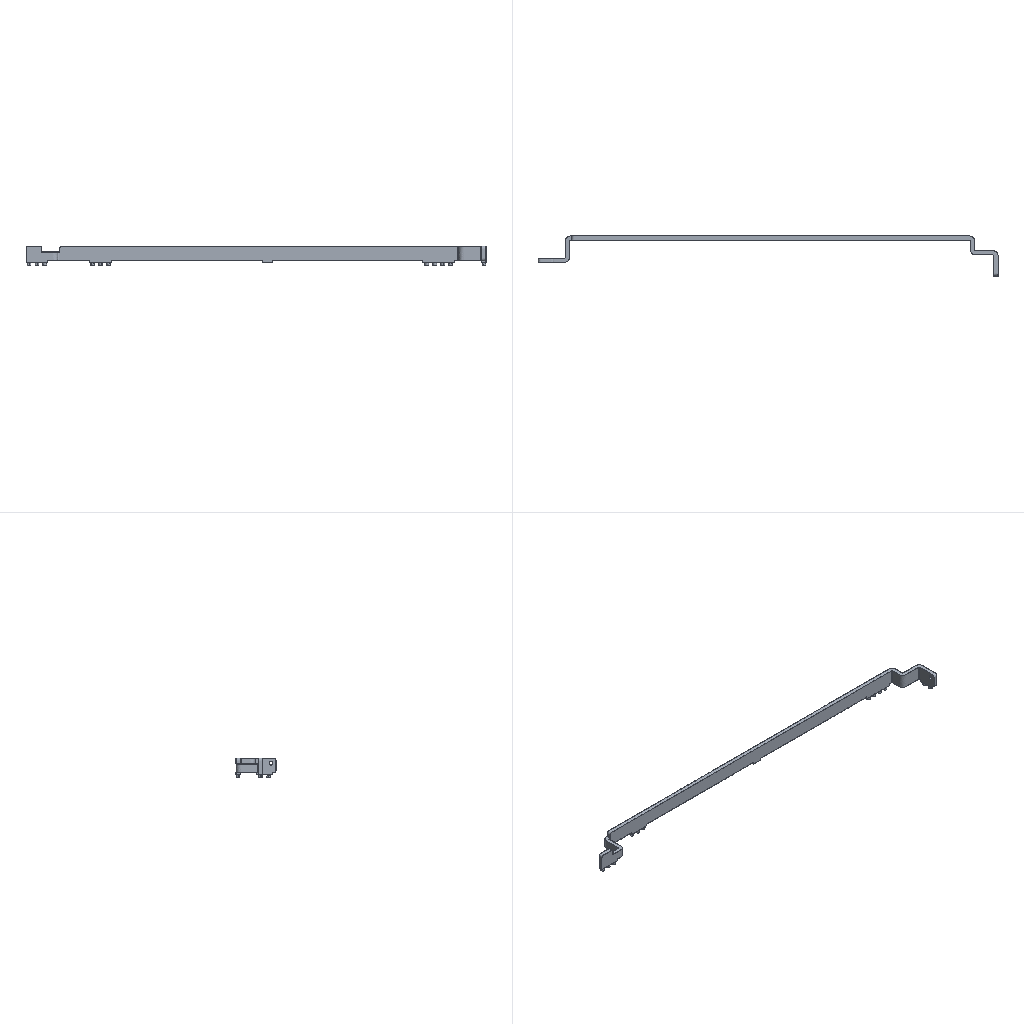Simulation study | ansys workbench
Set-up summary:
category,name,step,type,value,unit,region
solver,ansys_workbench
units,um-kg-s,,stated,"/units,uMKS"
analysis,LS1,,steady-state thermal
load_step,LS1,LS1,steady-state thermal,nsubst=1; time=1
mesh,nodes,,,149873
mesh,elements,,,151301
element_type,SOLID291,,,45869
element_type,227,,,30168
element_type,TARGE170,,,29349
element_type,CONTA174,,,29349
element_type,SURF152,,,16566
material,?,,E,3780,MPa
material,?,,nu,0.35
material,?,,density,1.16e-15,kg um^-3
material,?,,conductivity,200000,pW um^-1 C^-1
material,Copper Alloy,,E,110000,MPa
material,Copper Alloy,,nu,0.34
material,Copper Alloy,,density,8.3e-15,kg um^-3
material,Copper Alloy,,conductivity,4.01e+08,pW um^-1 C^-1
material,Copper Alloy,,specific_heat,3.85e+14,pJ kg^-1 C^-1
material,Copper Alloy,,cte,1.8e-05,C^-1
material,Copper Alloy,,permeability,1
material,Copper Alloy,,resistivity,1.548e-14
load,,LS1,force,0 [n=2],,node list
load,"Create ""______""",LS1,convection,20,,SURF152 #5
bc,,LS1,prescribed volt,[dofs=VOLT],,node list
contact,Contact Region,,bonded (always),element=CONTA174
constraint,ce,,,948
named_set,_CM38,,node,455
Ansys APDL input file, long lists of numbers shortened:
/batch
/config,noeldb,1     ! force off writing results to database
*get,_wallstrt,active,,time,wall
! ANSYS input file written by Workbench version 2021 R2
! File used for geometry attach:
/title,wbnew--______ (A5)
! ****** Begin Custom Load Command Snippet ******
/COM, ACT Extensions:
/COM,     LSDYNA, 2021.1
/COM,
! ****** End   Custom Load Command Snippet ******
*DIM,_wb_ProjectScratch_dir,string,248
_wb_ProjectScratch_dir(1) = ''
*DIM,_wb_SolverFiles_dir,string,248
_wb_SolverFiles_dir(1) = ''
*DIM,_wb_userfiles_dir,string,248
_wb_userfiles_dir(1) = ''
/com,--- Data in consistent uMKS units. See Solving Units in the help system for more information.
/units,uMKS
/nopr
/wb,file,start              !  signify a WB generated input file
/prep7
! Turn off shape checking because checks already performed inside WB mesher.
! See help system for more information.
SHPP,OFF,,NOWARN
ncnv,1,1e9             ! uMKS system, Increase DOF limit to 1e9
/nolist
etcon,set             ! allow ANSYS to choose best KEYOP's for 180x elements, resets any applicable keyopt to MAPDL defaults
/com,*********** Nodes for the whole assembly ***********
nblock,3,,164860
(1i9,3e20.9e3)
        1     8.444409090E+04     1.904694042E+04     7.400000000E+03
! (149872 more lines like these left out)
-1
/wb,elem,start            !  set before creation of elements
/com,*********** Elements for Body 1 "i24A7-2S - COATING" ***********
et,1,291
eblock,19,solid,,45869
(19i9)
        1        1        1        1        0        0        0        0       10        0    30169    57363    72055    62480    57436    73682   107343    73679    73678
! (91737 more lines like these left out)
-1
/com,*********** Elements for Body 2 "i24A7-2S" ***********
et,2,227,110
eblock,19,solid,,30168
(19i9)
        2        2        2        2        0        0        0        0       10        0        1     3967     9597     8304     8315    32140    53754    32137    32138
! (60335 more lines like these left out)
-1
/wb,elem,end               !  done creating elements
/com,*********** Send User Defined Coordinate System(s) ***********
csys,0
toffst,273.15,  ! Temperature offset from absolute zero
/com,*********** Set Reference Temperature ***********
tref,22.
/wb,mat,start              !  starting to send materials
/com,*********** Send Materials ***********
MP,DENS,1,1.16e-15,	! kg um^-3
MP,EX,1,3780,	! MPa
MP,NUXY,1,0.35,
MP,KXX,1,200000,	! pW um^-1 C^-1
Temperature = 'TEMP' ! Temperature
MP,DENS,2,8.3e-15,	! kg um^-3
MP,ALPX,2,1.8e-05,	! C^-1
MP,C,2,385000000000000,	! pJ kg^-1 C^-1
MP,KXX,2,401000000,	! pW um^-1 C^-1
MPTEMP,,,,,,,,
MPTEMP,1,0
MPTEMP,2,20
MPTEMP,3,100
MPDATA,RSVX,2, ,1.548e-14,1.694e-14,2.277e-14,	! Tohm um
MPTEMP,,,,,,,,
MP,EX,2,110000,	! MPa
MP,NUXY,2,0.34,
MP,MURX,2,1,
/wb,mat,end                !  done sending materials
!************************* Model Summary ********************
!i24A7-2S - COATING,	环氧树脂,	matid,	1
!i24A7-2S,	铜合金,	matid,	2
!************************* End Model Summary ********************
! get the diagonal of the bounding box. Needed later for other things
*get,_xmin,node,,mnloc,x
*get,_ymin,node,,mnloc,y
*get,_zmin,node,,mnloc,z
*get,_xmax,node,,mxloc,x
*get,_ymax,node,,mxloc,y
*get,_zmax,node,,mxloc,z
_ASMDIAG=(_xmax-_xmin)*(_xmax-_xmin)+(_ymax-_ymin)*(_ymax-_ymin)+(_zmax-_zmin)*(_zmax-_zmin)
_ASMDIAG=SQRT(_ASMDIAG)
/wb,contact,start          !  starting to send contact
/com,*********** Create Contact "接触区域" ***********
/com,            Real Constant Set For Above Contact Is 4 & 3
*set,tid,4
*set,cid,3
r,tid
r,cid
et,tid,170
et,cid,174
eblock,10,,,15039
(15i9)
   122828        4        4        4        0    60070    60066    60071    60071    91609    91610    60071    91632
! (15038 more lines like these left out)
-1
eblock,10,,,15039
(15i9)
   137867        3        3        3        0    60070    60066    60071    60071    91609    91610    60071    91632
! (15038 more lines like these left out)
-1
eblock,10,,,14310
(15i9)
   152906        3        4        3        0      268      264      267      267    11334    11333      267    11360
! (14309 more lines like these left out)
-1
eblock,10,,,14310
(15i9)
   167216        4        3        4        0      268      264      267      267    11334    11333      267    11360
! (14309 more lines like these left out)
-1
keyo,cid,8,2               ! auto create asymmetric contact (from Program Controlled setting)
keyo,cid,10,0              ! adjust contact stiffness each NR iteration (from Program Controlled setting)
keyo,cid,12,5              ! bonded always
keyo,cid,18,1              ! small sliding turned on by application
keyo,cid,2,0               ! augmented Lagrange (from Program Controlled setting)
keyo,cid,4,0               ! on Gauss point (from Program Controlled setting)
keyo,cid,9,1               ! ignore initial gaps/penetration
keyo,cid,7,0               ! No Prediction
rmod,tid,3,10.      ! FKN
rmod,tid,5,0.       ! ICONT
rmod,tid,6,0.       ! PINB
rmod,tid,10,0.      ! CNOF
rmod,tid,12,0.      ! FKT
rmod,tid,36,29      ! WB DSID
rmod,cid,3,10.      ! FKN
rmod,cid,5,0.       ! ICONT
rmod,cid,6,0.       ! PINB
rmod,cid,10,0.      ! CNOF
rmod,cid,12,0.      ! FKT
rmod,cid,36,29      ! WB DSID
*set,_maxkxx,4010000000000.
rmod,cid,14,_maxkxx/_ASMDIAG         ! TCC, Divide by Length since Traction Based
rmod,tid,14,_maxkxx/_ASMDIAG      ! TCC, Divide by Length since Traction Based
keyo,cid,1,2     ! Pure thermal contact
nsel,all
esel,all
/wb,contact,end            !  done creating contacts
/golist
/wb,load,start             !  starting to send loads
/com,*********** Create Voltage "__" ***********
CMBLOCK,_CM38   ,NODE,      455
(8i10)
       140       141       142       143       144       145       146       147
! (56 more lines like these left out)
/com,*********** Create Current ***********
/com,*********** Create Current ***********
fcum,add                   ! add nodal forces up (needed in case have loads on the same edge,vertex)
fcum                       ! reset default on fcum command since done sending WB F loads
/com,*********** Create "______" ***********
et,5,152
eblock,10,,,16566
(15i9)
   181526        5        5        5        0    57519    57520    59741    59741    74470    74476    59741    74472
! (16565 more lines like these left out)
-1
esel,s,type,,5
keyop,5,8,2.
keyop,5,13,0
esel,all
/gst,on,on
fini
*get,_numnode,node,0,count
*get,_numelem,elem,0,count
*get, _MAXELEMNUM, elem, 0, NUM, MAX
*get, _MAXNODENUM, node, 0, NUM, MAX
*get, _MAXELEMTYPE, etyp, 0, NUM, MAX
*get, _MAXREALCONST, real, 0, NUM, MAX
/go
/wb,load,end               !  done creating loads
/com,--- Number of total nodes = %_numnode%
/com,--- Number of contact elements = 75264
/com,--- Number of spring elements = 0
/com,--- Number of bearing elements = 0
/com,--- Number of solid elements = 76037
/com,--- Number of condensed parts = 0
/com,--- Number of total elements = %_numelem%
*get,_wallbsol,active,,time,wall
/com,****************************************************************************
/com,*************************    SOLUTION       ********************************
/com,****************************************************************************
/solu
antype,0                   ! static analysis
!eqsl,sparse               ! using sparse solver which is default so no eqsl command needed
cntr,print,1               ! print out contact info and also make no initial contact an error
dmpoption,emat,no             ! Don't combine emat file for DANSYS
dmpoption,esav,no             ! Don't combine esav file for DANSYS
/com,****************************************************
/com,******************* SOLVE FOR LS 1 OF 1****************
d,_CM38,volt,0.
nsel,all
f,23,amps,140000000000000
ce,next,0.,23,volt,-1.,24,volt,1.
ce,next,0.,23,volt,-1.,25,volt,1.
! (295 more lines like these left out)
f,61,amps,70000000000000.
ce,next,0.,61,volt,-1.,62,volt,1.
ce,next,0.,61,volt,-1.,63,volt,1.
! (649 more lines like these left out)
/nopr
/gopr
esel,s,type,,5
nsle
sf,all,conv,20.,40.
nsel,all
esel,all
autots,on
nsub,1,10,1
time,1.
outres,erase
outres,all,none
outres,nsol,all
outres,rsol,all
outres,eangl,all
outres,veng,all
outres,fflux,all
outres,fgrad,all
outres,eheat,all
outres,cont,all
/nopr
esel,s,type,,5
cm,_elmisc,elem
esel,all
/gopr
outres,misc,all,_elmisc
cnvtol,heat,,.001,,1000000.   ! Program Controlled. Set MINREF equivalent of 1e-6 Watts
cnvtol,amps,,.001,,1000000.   ! Program Controlled. Set MINREF equivalent of 1e-6 A
neqit,1000
! *********** WB SOLVE COMMAND ***********
! check interactive state
*get,ANSINTER_,active,,int
*if,ANSINTER_,ne,0,then
/eof
*endif
solve
/com *************** Write FE CONNECTORS *********
CEWRITE,file,ce,,INTE
/com,****************************************************
/com,*************** FINISHED SOLVE FOR LS 1 *************
*get,_wallasol,active,,time,wall
/post1
xmlo,ENCODING,ISO-8859-1
xmlo,parm
/xml,parm,xml
fini
/gopr
*get,_walldone,active,,time,wall
_preptime=(_wallbsol-_wallstrt)*3600
_solvtime=(_wallasol-_wallbsol)*3600
_posttime=(_walldone-_wallasol)*3600
_totaltim=(_walldone-_wallstrt)*3600
*get,_dlbratio,active,0,solu,dlbr
*get,_combtime,active,0,solu,comb
*get,_ssmode,active,0,solu,ssmm
*get,_ndofs,active,0,solu,ndof
/com,--- Total number of nodes = %_numnode%
/com,--- Total number of elements = %_numelem%
/com,--- Element load balance ratio = %_dlbratio%
/com,--- Time to combine distributed files = %_combtime%
/com,--- Sparse memory mode = %_ssmode%
/com,--- Number of DOF = %_ndofs%
/wb,file,end               ! done with WB generated input
Results summary:
result,analyses[0].index,,,1
result,analyses[0].system,,,SYS
result,analyses[0].deck,,,deck.dat
result,analyses[0].solve_status,,,completed
result,analyses[0].analysis_type,,,static
result,analyses[0].physics,,,mechanical
result,analyses[0].unit_system,,,"UMKS: um, kg, uN, s, V, mA, degC"
result,analyses[0].n_sets,,,1
result,analyses[0].load_steps[0].set,set=1,,1
result,analyses[0].load_steps[0].time_or_freq,set=1,,1
result,analyses[0].load_steps[0].max_temperature,set=1,,59.979
result,analyses[0].load_steps[0].min_temperature,set=1,,53.623
result,geometry_export[0][0],,,.step
result,geometry_export[0][1],,,ok
result,geometry_export[0][2],,,2